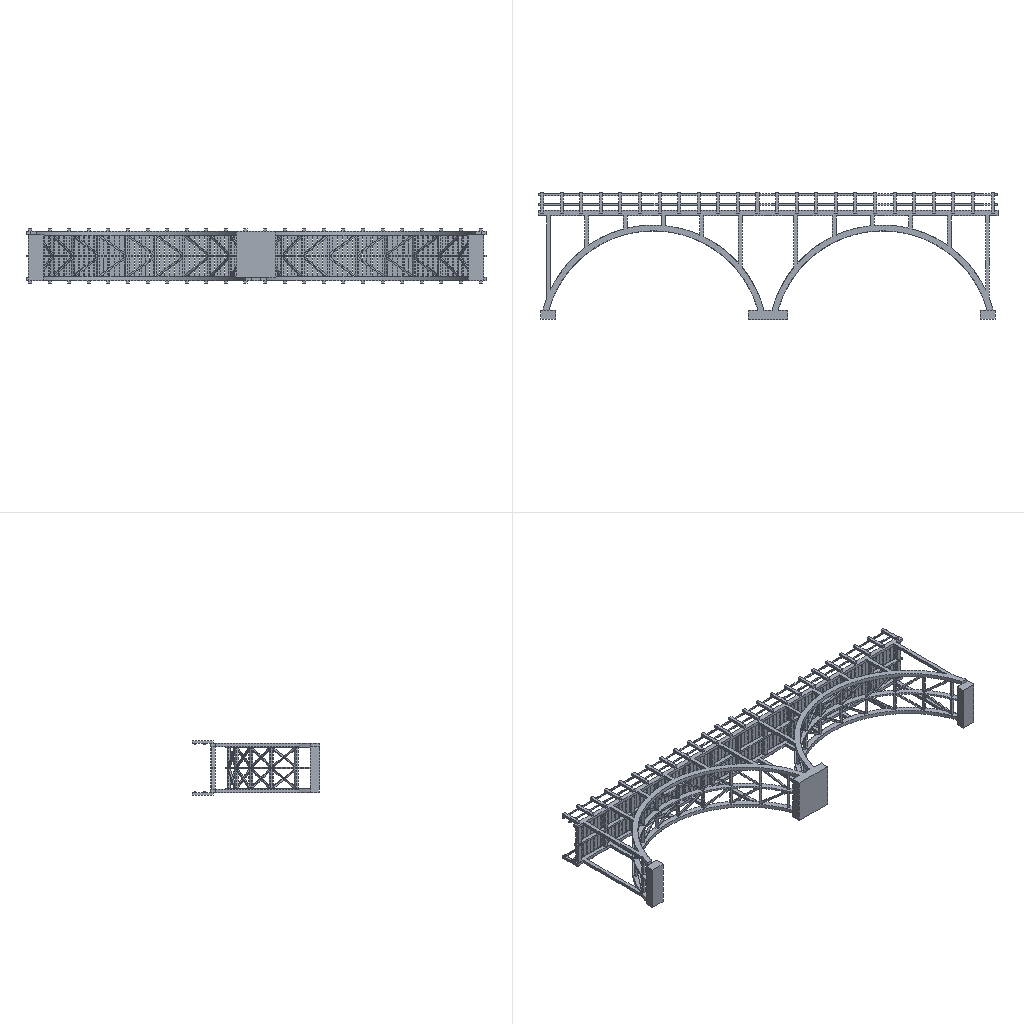Simulation study | ansys workbench
Set-up summary:
category,name,step,type,value,unit,region
solver,ansys_workbench
units,SI m-kg-s (Pa),,stated,"/units,MKS"
analysis,LS1,,static
load_step,LS1,LS1,static,nsubst=1; time=1
mesh,nodes,,,700343
mesh,elements,,,393800
element_type,SOLID187,,,391290
element_type,SURF154,,,2510
material,Structural Steel,,E,2e+11,Pa
material,Structural Steel,,nu,0.3
material,Structural Steel,,density,7850,kg m^-3
material,Structural Steel,,conductivity,60.5,W m^-1 C^-1
material,Structural Steel,,specific_heat,434,J kg^-1 C^-1
material,Structural Steel,,cte,1.2e-05,C^-1
material,Structural Steel,,permeability,10000
material,Structural Steel,,resistivity,1.7e-07,kg m^3 A^-2 s^-3
load,Define Force Using Surface Effect Elements,LS1,surface-effect pres face 2,-8072.93,,SURF154 #2
bc,Fixed Supports,model,fixed,[dofs=ALL],,_FIXEDSU
named_set,_FIXEDSU,,node,5991
Ansys APDL input file, long lists of numbers shortened:
/batch
/config,noeldb,1     ! force off writing results to database
*get,_wallstrt,active,,time,wall
! ANSYS input file written by Workbench version 2024 R2
! File used for geometry attach:
/title,wbnew--____ (A5)
! ****** Begin Custom Load Command Snippet ******
/COM, ACT Extensions:
/COM,     LSDYNA, 2024.2
/COM,/COM,     ANSYSMotion, 2024.2
/COM,
! ****** End   Custom Load Command Snippet ******
*DIM,_wb_ProjectScratch_dir,string,248
_wb_ProjectScratch_dir(1) = ''
*DIM,_wb_SolverFiles_dir,string,248
_wb_SolverFiles_dir(1) = ''
*DIM,_wb_userfiles_dir,string,248
_wb_userfiles_dir(1) = ''
/com,--- Data in consistent MKS units. See Solving Units in the help system for more information.
/units,MKS
/nopr
/wb,file,start              !  signify a WB generated input file
/prep7
! Turn off shape checking because checks already performed inside WB mesher.
! See help system for more information.
SHPP,OFF,,NOWARN
/nolist
etcon,set             ! allow ANSYS to choose best KEYOP's for 180x elements, resets any applicable keyopt to MAPDL defaults
/com,*********** Nodes for the whole assembly ***********
nblock,3,,770377
(1i9,3e20.9e3)
        1     0.000000000E+00     1.017388191E+00     1.524000000E-01
! (700342 more lines like these left out)
-1
/wb,elem,start            !  set before creation of elements
/com,*********** Elements for Body 1 'Part1-FreeParts' ***********
et,1,187
eblock,19,solid,,391290
(19i9)
        1        1        1        1        0        0        0        0       10        0        1    79766    94547   113068   107334   557799   625999   557803   557802
! (782579 more lines like these left out)
-1
/wb,elem,end               !  done creating elements
/com,*********** Send User Defined Coordinate System(s) ***********
csys,0
toffst,273.15,      ! Temperature offset from absolute zero
/com,*********** Set Reference Temperature ***********
tref,22.
/wb,mat,start              !  starting to send materials
/com,*********** Send Materials ***********
Temperature = 'TEMP' ! Temperature
MP,DENS,1,7850,	! kg m^-3
MP,ALPX,1,1.2e-05,	! C^-1
MP,C,1,434,	! J kg^-1 C^-1
MP,KXX,1,60.5,	! W m^-1 C^-1
MP,RSVX,1,1.7e-07,	! kg m^3 A^-2 s^-3
MP,EX,1,200000000000,	! Pa
MP,NUXY,1,0.3,
MP,MURX,1,10000,
/wb,mat,end                !  done sending materials
!************************* Model Summary ********************
!Part1-FreeParts,	结构钢,	matid,	1
!************************* End Model Summary ********************
! get the diagonal of the bounding box. Needed later for other things
*get,_xmin,node,,mnloc,x
*get,_ymin,node,,mnloc,y
*get,_zmin,node,,mnloc,z
*get,_xmax,node,,mxloc,x
*get,_ymax,node,,mxloc,y
*get,_zmax,node,,mxloc,z
_ASMDIAG=(_xmax-_xmin)*(_xmax-_xmin)+(_ymax-_ymin)*(_ymax-_ymin)+(_zmax-_zmin)*(_zmax-_zmin)
_ASMDIAG=SQRT(_ASMDIAG)
/wb,contact,start          !  starting to send contact
/wb,contact,end            !  done creating contacts
/golist
/wb,load,start             !  starting to send loads
/com,*********** Fixed Supports ***********
CMBLOCK,_FIXEDSU,NODE,     5991
(8i10)
      5096      5103      5104      5105      5106      5107      5108      5109
! (748 more lines like these left out)
cmsel,s,_FIXEDSU
d,all,all
nsel,all
/com,*********** Define Force Using Surface Effect Elements ***********
local,12,0,0.,0.,0.,0.,0.,0.
csys,0
et,2,154
mat,2
eblock,10,,,2510
(15i9)
   556233        2        2        2       12     4815     4816    13963    13963   142476   142480    13963   142478
! (2509 more lines like these left out)
-1
esel,s,type,,2
keyop,2,2,1         ! Apply load in local coordinate system
keyop,2,7,1         ! Use original area so load is constant in large deformation
esel,all
/gst,on,on
fini
*get,_numnode,node,0,count
*get,_numelem,elem,0,count
*get, _MAXELEMNUM, elem, 0, NUM, MAX
*get, _MAXNODENUM, node, 0, NUM, MAX
*get, _MAXELEMTYPE, etyp, 0, NUM, MAX
*get, _MAXREALCONST, rcon, 0, NUM, MAX
/go
/wb,load,end               !  done creating loads
/com,--- Number of total nodes = %_numnode%
/com,--- Number of contact elements = 2510
/com,--- Number of spring elements = 0
/com,--- Number of bearing elements = 0
/com,--- Number of solid elements = 391290
/com,--- Number of condensed parts = 0
/com,--- Number of total elements = %_numelem%
*get,_wallbsol,active,,time,wall
/com,****************************************************************************
/com,*************************    SOLUTION       ********************************
/com,****************************************************************************
/solu
antype,0                   ! static analysis
_thickRatio=  1     ! Ratio of thick parts in the model
eqsl,pcg,1e-8,,,,,,1
cntr,print,1               ! print out contact info and also make no initial contact an error
cncheck,dmp		!	Enable program controlled contact splitting for distributed memory parallel run
dmpoption,emat,no             ! Don't combine emat file for DANSYS
dmpoption,esav,no             ! Don't combine esav file for DANSYS
nldiag,cont,iter           ! print out contact info each equilibrium iteration
rescontrol,,none                 ! Do not keep any restart files
/com,****************************************************
/com,******************* SOLVE FOR LS 1 OF 1 ****************
esel,s,type,,2
nsle
sfe,all,1,pres,1,0.
sfe,all,2,pres,1,-8072.933
sfe,all,3,pres,1,0.
nsel,all
esel,all
/nopr
/gopr
nsub,1,1,1
time,1.
outres,erase
outres,all,none
outres,nsol,all,
outres,rsol,all
outres,eangl,all
outres,etmp,all
outres,veng,all
outres,strs,all,
outres,epel,all,
outres,eppl,all,
outres,cont,all,
! *********** WB SOLVE COMMAND ***********
! check interactive state
*get,ANSINTER_,active,,int
*if,ANSINTER_,ne,0,then
/eof
*endif
solve
/com *************** Write FE CONNECTORS *********
CEWRITE,file,ce,,INTE
/com,****************************************************
/com,*************** FINISHED SOLVE FOR LS 1 *************
*get,_wallasol,active,,time,wall
/nopr
*get,_numnode,node,0,count
*get,_numelem,elem,0,count
*get, _MAXELEMNUM, elem, 0, NUM, MAX
*get, _MAXNODENUM, node, 0, NUM, MAX,,,INTERNAL
*get, _MAXELEMTYPE, etyp, 0, NUM, MAX
*get, _MAXREALCONST, rcon, 0, NUM, MAX
*get,_NSOLTHREADS,active,0,ntfs
*get,_NSOLPROCESSES,active,0,npfs
/gopr
*get,_PCGITER,active,,solu,cgiter
/post1
xmlo,ENCODING,ISO-8859-1
xmlo,parm
/xml,parm,xml
fini
/gopr
*get,_walldone,active,,time,wall
_preptime=(_wallbsol-_wallstrt)*3600
_solvtime=(_wallasol-_wallbsol)*3600
_posttime=(_walldone-_wallasol)*3600
_totaltim=(_walldone-_wallstrt)*3600
*get,_dlbratio,active,0,solu,dlbr
*get,_combtime,active,0,solu,comb
*get,_ssmode,active,0,solu,ssmm
*get,_ndofs,active,0,solu,ndof
*get,_sol_end_time,active,0,set,time
*if,_sol_end_time,eq,1.,then
/fclean				!clean distributed files
*endif
/com,--- Total number of nodes = %_numnode%
/com,--- Total number of elements = %_numelem%
/com,--- Element load balance ratio = %_dlbratio%
/com,--- Time to combine distributed files = %_combtime%
/com,--- Sparse memory mode = %_ssmode%
/com,--- Number of DOF = %_ndofs%
/wb,file,end               ! done with WB generated input
Results summary:
result,analyses[0].index,,,1
result,analyses[0].system,,,SYS
result,analyses[0].deck,,,deck.dat
result,analyses[0].solve_status,,,completed
result,analyses[0].analysis_type,,,static
result,analyses[0].physics,,,mechanical
result,analyses[0].unit_system,,,"MKS: m, kg, N, s, V, A, degC"
result,analyses[0].n_sets,,,1
result,analyses[0].load_steps[0].set,set=1,,1
result,analyses[0].load_steps[0].time_or_freq,set=1,,1
result,analyses[0].load_steps[0].max_displacement_magnitude,set=1,,2.74407e-05
result,analyses[0].load_steps[0].max_von_mises_nodal,set=1,,1.72883e+06
result,analyses[0].load_steps[0].reaction_force_sum_xyz[1],set=1,,5.04929e-06
result,analyses[0].load_steps[0].reaction_force_sum_xyz[2],set=1,,100000
result,analyses[0].load_steps[0].reaction_force_sum_xyz[3],set=1,,6.5363e-05